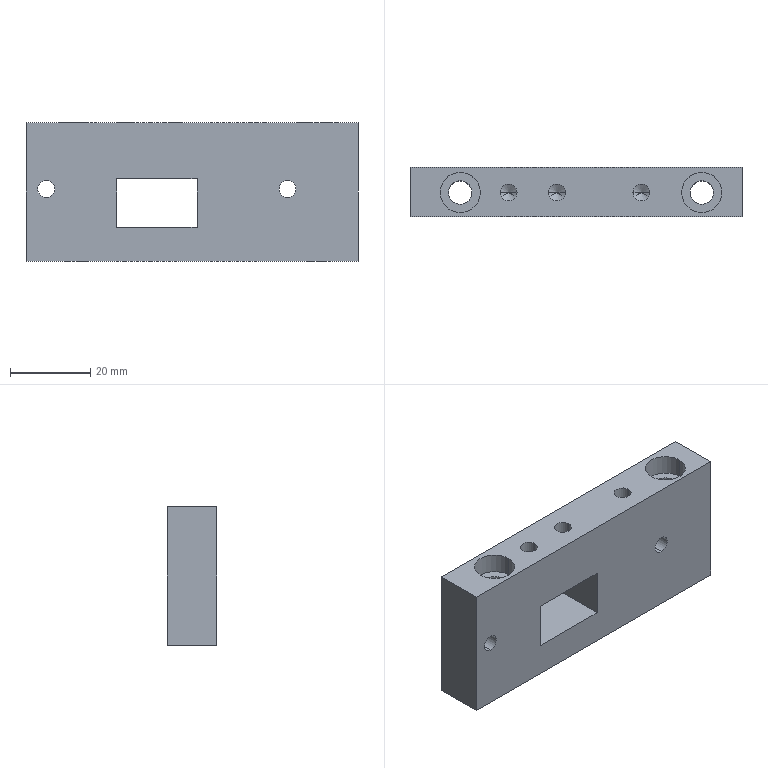Part | STEP file | secondary slingshot input side block 1 | 1 solid | 36 faces | box 82.5 x 12.3 x 34.5 mm | volume 28839 mm3 | cylinder 18 | plane 12 | cone 6 | commonest cylinder face diameters 4.2 x10 5.8 x4 10 x4